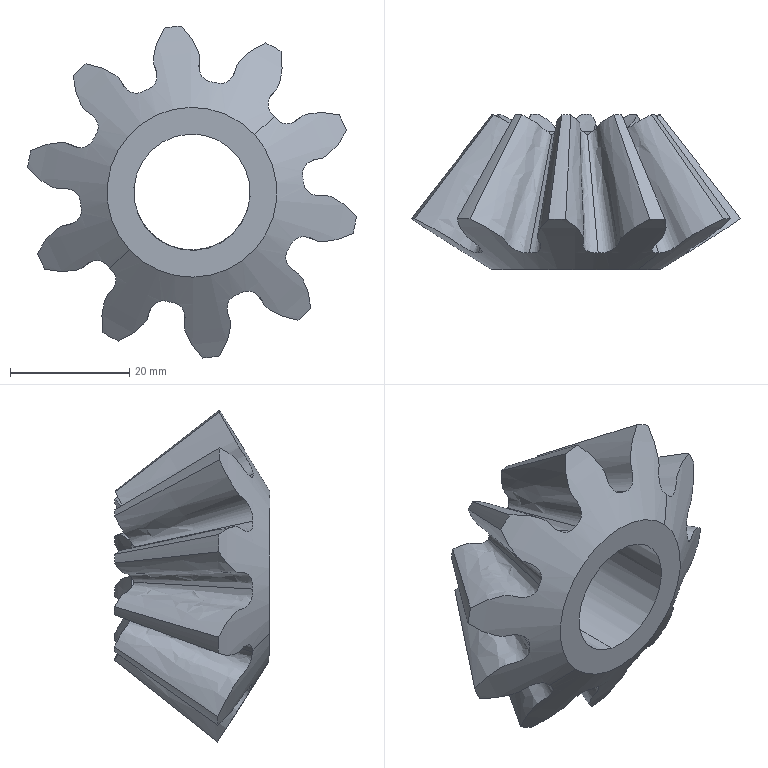Part | NX | features BREP 1 | 1 solid | 45 faces | box 55.15 x 26.094 x 55.633 mm | volume 18314 mm3 | cone 22 | spline 20 | cylinder 2 | plane 1 | commonest cylinder face diameters 19.5 x2